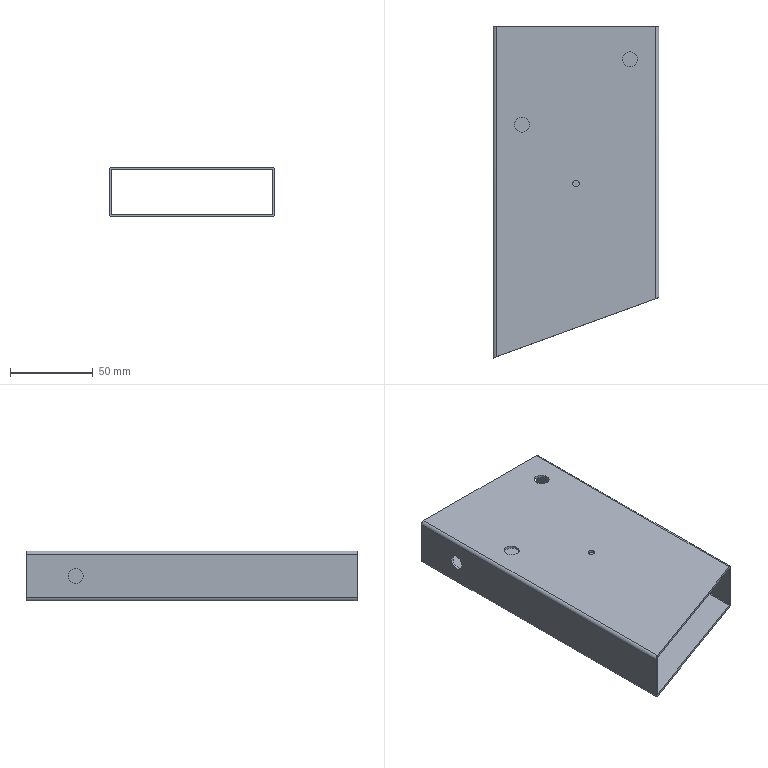Part | STEP file | PN_0021 | 1 solid | 22 faces | box 100 x 200 x 30 mm | volume 68376 mm3 | cylinder 12 | plane 10 | commonest cylinder face diameters 4 x5 1 x4 9 x3